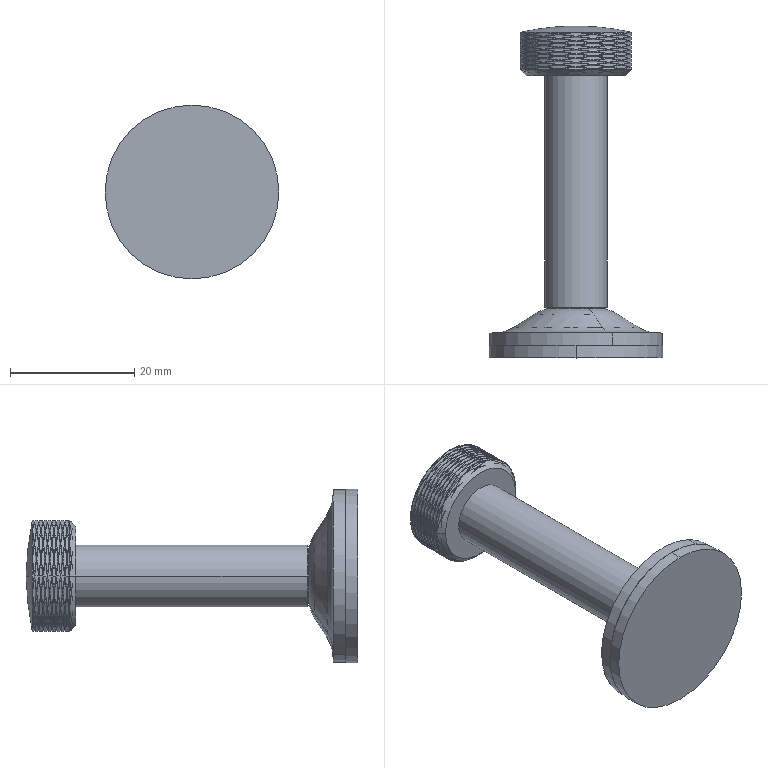Part | SolidWorks | 3 solids | 1023 faces | box 28 x 53.48 x 28 mm | volume 7166 mm3 | spline 760 | cylinder 212 | cone 22 | plane 19 | torus 8 | sphere 2 | commonest cylinder face diameters 18 x200 3.3 x2 5.2 x2 5.6 x2 10 x2 27.8 x2